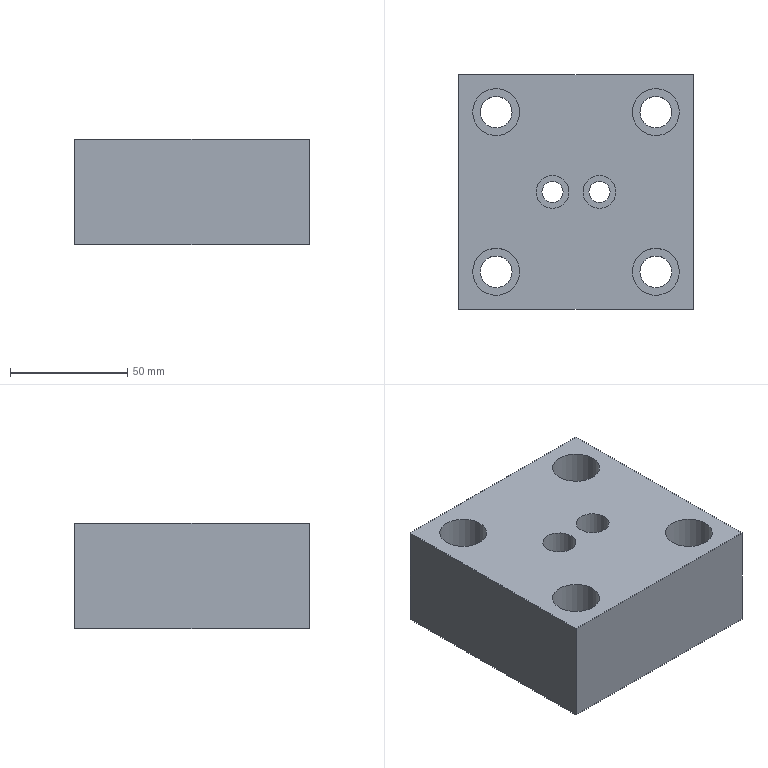Part | STEP file | lll_id554_x_t | 1 solid | 26 faces | box 100 x 100 x 45 mm | volume 329147 mm3 | plane 13 | cylinder 13 | commonest cylinder face diameters 13.509 x4 20.008 x4 9 x2 14 x2 65.2 x1
STEP:
#1=CARTESIAN_POINT('',(1525.035,-187.,246.5));
#2=VERTEX_POINT('',#1);
#3=CARTESIAN_POINT('',(1492.435,-187.,246.5));
#4=DIRECTION('',(0.,0.,1.));
#5=DIRECTION('',(1.,0.,0.));
#6=AXIS2_PLACEMENT_3D('',#3,#4,#5);
#7=CIRCLE('',#6,32.6);
#8=EDGE_CURVE('',#2,#2,#7,.T.);
#9=ORIENTED_EDGE('',*,*,#8,.F.);
#10=EDGE_LOOP('',(#9));
#11=FACE_BOUND('',#10,.T.);
#12=CARTESIAN_POINT('',(1486.935,-187.,246.5));
#13=VERTEX_POINT('',#12);
#14=CARTESIAN_POINT('',(1482.435,-187.,246.5));
#15=DIRECTION('',(0.,0.,1.));
#16=DIRECTION('',(1.,0.,0.));
#17=AXIS2_PLACEMENT_3D('',#14,#15,#16);
#18=CIRCLE('',#17,4.5);
#19=EDGE_CURVE('',#13,#13,#18,.T.);
#20=ORIENTED_EDGE('',*,*,#19,.T.);
#21=EDGE_LOOP('',(#20));
#22=FACE_BOUND('',#21,.T.);
#23=CARTESIAN_POINT('',(1506.935,-187.,246.5));
#24=VERTEX_POINT('',#23);
#25=CARTESIAN_POINT('',(1502.435,-187.,246.5));
#26=DIRECTION('',(0.,0.,-1.));
#27=DIRECTION('',(1.,0.,0.));
#28=AXIS2_PLACEMENT_3D('',#25,#26,#27);
#29=CIRCLE('',#28,4.5);
#30=EDGE_CURVE('',#24,#24,#29,.T.);
#31=ORIENTED_EDGE('',*,*,#30,.F.);
#32=EDGE_LOOP('',(#31));
#33=FACE_BOUND('',#32,.T.);
#34=CARTESIAN_POINT('',(1477.135,-187.,246.5));
#35=DIRECTION('',(0.,0.,1.));
#36=DIRECTION('',(1.,0.,0.));
#37=AXIS2_PLACEMENT_3D('',#34,#35,#36);
#38=PLANE('',#37);
#39=ADVANCED_FACE('',(#11,#22,#33),#38,.F.);
#40=CARTESIAN_POINT('',(1509.435,-187.,267.5));
#41=VERTEX_POINT('',#40);
#42=CARTESIAN_POINT('',(1502.435,-187.,267.5));
#43=DIRECTION('',(0.,0.,1.));
#44=DIRECTION('',(1.,0.,0.));
#45=AXIS2_PLACEMENT_3D('',#42,#43,#44);
#46=CIRCLE('',#45,7.);
#47=EDGE_CURVE('',#41,#41,#46,.T.);
#48=ORIENTED_EDGE('',*,*,#47,.F.);
#49=EDGE_LOOP('',(#48));
#50=FACE_BOUND('',#49,.T.);
#51=CARTESIAN_POINT('',(1489.435,-187.,267.5));
#52=VERTEX_POINT('',#51);
#53=CARTESIAN_POINT('',(1482.435,-187.,267.5));
#54=DIRECTION('',(0.,0.,1.));
#55=DIRECTION('',(1.,0.,0.));
#56=AXIS2_PLACEMENT_3D('',#53,#54,#55);
#57=CIRCLE('',#56,7.);
#58=EDGE_CURVE('',#52,#52,#57,.T.);
#59=ORIENTED_EDGE('',*,*,#58,.F.);
#60=EDGE_LOOP('',(#59));
#61=FACE_BOUND('',#60,.T.);
#62=CARTESIAN_POINT('',(1536.439,-153.,267.5));
#63=VERTEX_POINT('',#62);
#64=CARTESIAN_POINT('',(1526.435,-153.,267.5));
#65=DIRECTION('',(0.,0.,-1.));
#66=DIRECTION('',(1.,0.,0.));
#67=AXIS2_PLACEMENT_3D('',#64,#65,#66);
#68=CIRCLE('',#67,10.004);
#69=EDGE_CURVE('',#63,#63,#68,.T.);
#70=ORIENTED_EDGE('',*,*,#69,.T.);
#71=EDGE_LOOP('',(#70));
#72=FACE_BOUND('',#71,.T.);
#73=CARTESIAN_POINT('',(1468.439,-221.,267.5));
#74=VERTEX_POINT('',#73);
#75=CARTESIAN_POINT('',(1458.435,-221.,267.5));
#76=DIRECTION('',(0.,0.,-1.));
#77=DIRECTION('',(1.,0.,0.));
#78=AXIS2_PLACEMENT_3D('',#75,#76,#77);
#79=CIRCLE('',#78,10.004);
#80=EDGE_CURVE('',#74,#74,#79,.T.);
#81=ORIENTED_EDGE('',*,*,#80,.T.);
#82=EDGE_LOOP('',(#81));
#83=FACE_BOUND('',#82,.T.);
#84=CARTESIAN_POINT('',(1542.435,-137.,267.5));
#85=VERTEX_POINT('',#84);
#86=CARTESIAN_POINT('',(1542.435,-237.,267.5));
#87=VERTEX_POINT('',#86);
#88=CARTESIAN_POINT('',(1542.435,-187.,267.5));
#89=DIRECTION('',(0.,-1.,0.));
#90=VECTOR('',#89,1.);
#91=LINE('',#88,#90);
#92=EDGE_CURVE('',#85,#87,#91,.T.);
#93=ORIENTED_EDGE('',*,*,#92,.F.);
#94=CARTESIAN_POINT('',(1442.435,-137.,267.5));
#95=VERTEX_POINT('',#94);
#96=CARTESIAN_POINT('',(1492.435,-137.,267.5));
#97=DIRECTION('',(1.,0.,0.));
#98=VECTOR('',#97,1.);
#99=LINE('',#96,#98);
#100=EDGE_CURVE('',#95,#85,#99,.T.);
#101=ORIENTED_EDGE('',*,*,#100,.F.);
#102=CARTESIAN_POINT('',(1442.435,-237.,267.5));
#103=VERTEX_POINT('',#102);
#104=CARTESIAN_POINT('',(1442.435,-187.,267.5));
#105=DIRECTION('',(0.,1.,0.));
#106=VECTOR('',#105,1.);
#107=LINE('',#104,#106);
#108=EDGE_CURVE('',#103,#95,#107,.T.);
#109=ORIENTED_EDGE('',*,*,#108,.F.);
#110=CARTESIAN_POINT('',(1492.435,-237.,267.5));
#111=DIRECTION('',(-1.,0.,0.));
#112=VECTOR('',#111,1.);
#113=LINE('',#110,#112);
#114=EDGE_CURVE('',#87,#103,#113,.T.);
#115=ORIENTED_EDGE('',*,*,#114,.F.);
#116=EDGE_LOOP('',(#93,#101,#109,#115));
#117=FACE_BOUND('',#116,.T.);
#118=CARTESIAN_POINT('',(1468.439,-153.,267.5));
#119=VERTEX_POINT('',#118);
#120=CARTESIAN_POINT('',(1458.435,-153.,267.5));
#121=DIRECTION('',(0.,0.,-1.));
#122=DIRECTION('',(1.,0.,0.));
#123=AXIS2_PLACEMENT_3D('',#120,#121,#122);
#124=CIRCLE('',#123,10.004);
#125=EDGE_CURVE('',#119,#119,#124,.T.);
#126=ORIENTED_EDGE('',*,*,#125,.T.);
#127=EDGE_LOOP('',(#126));
#128=FACE_BOUND('',#127,.T.);
#129=CARTESIAN_POINT('',(1536.439,-221.,267.5));
#130=VERTEX_POINT('',#129);
#131=CARTESIAN_POINT('',(1526.435,-221.,267.5));
#132=DIRECTION('',(0.,0.,-1.));
#133=DIRECTION('',(1.,0.,0.));
#134=AXIS2_PLACEMENT_3D('',#131,#132,#133);
#135=CIRCLE('',#134,10.004);
#136=EDGE_CURVE('',#130,#130,#135,.T.);
#137=ORIENTED_EDGE('',*,*,#136,.T.);
#138=EDGE_LOOP('',(#137));
#139=FACE_BOUND('',#138,.T.);
#140=CARTESIAN_POINT('',(1492.435,-187.,267.5));
#141=DIRECTION('',(0.,0.,1.));
#142=DIRECTION('',(1.,0.,0.));
#143=AXIS2_PLACEMENT_3D('',#140,#141,#142);
#144=PLANE('',#143);
#145=ADVANCED_FACE('',(#50,#61,#72,#83,#117,#128,#139),#144,.T.);
#146=CARTESIAN_POINT('',(1525.035,-187.,222.5));
#147=VERTEX_POINT('',#146);
#148=CARTESIAN_POINT('',(1492.435,-187.,222.5));
#149=DIRECTION('',(0.,0.,1.));
#150=DIRECTION('',(1.,0.,0.));
#151=AXIS2_PLACEMENT_3D('',#148,#149,#150);
#152=CIRCLE('',#151,32.6);
#153=EDGE_CURVE('',#147,#147,#152,.T.);
#154=ORIENTED_EDGE('',*,*,#153,.F.);
#155=EDGE_LOOP('',(#154));
#156=FACE_BOUND('',#155,.T.);
#157=ORIENTED_EDGE('',*,*,#8,.T.);
#158=EDGE_LOOP('',(#157));
#159=FACE_BOUND('',#158,.T.);
#160=CARTESIAN_POINT('',(1492.435,-187.,246.5));
#161=DIRECTION('',(0.,0.,-1.));
#162=DIRECTION('',(-1.,0.,0.));
#163=AXIS2_PLACEMENT_3D('',#160,#161,#162);
#164=CYLINDRICAL_SURFACE('',#163,32.6);
#165=ADVANCED_FACE('',(#156,#159),#164,.F.);
#166=CARTESIAN_POINT('',(1442.435,-137.,222.5));
#167=VERTEX_POINT('',#166);
#168=CARTESIAN_POINT('',(1542.435,-137.,222.5));
#169=VERTEX_POINT('',#168);
#170=CARTESIAN_POINT('',(1492.435,-137.,222.5));
#171=DIRECTION('',(1.,0.,0.));
#172=VECTOR('',#171,1.);
#173=LINE('',#170,#172);
#174=EDGE_CURVE('',#167,#169,#173,.T.);
#175=ORIENTED_EDGE('',*,*,#174,.F.);
#176=CARTESIAN_POINT('',(1442.435,-137.,78.6));
#177=DIRECTION('',(0.,0.,1.));
#178=VECTOR('',#177,1.);
#179=LINE('',#176,#178);
#180=EDGE_CURVE('',#167,#95,#179,.T.);
#181=ORIENTED_EDGE('',*,*,#180,.T.);
#182=ORIENTED_EDGE('',*,*,#100,.T.);
#183=CARTESIAN_POINT('',(1542.435,-137.,78.6));
#184=DIRECTION('',(0.,0.,1.));
#185=VECTOR('',#184,1.);
#186=LINE('',#183,#185);
#187=EDGE_CURVE('',#169,#85,#186,.T.);
#188=ORIENTED_EDGE('',*,*,#187,.F.);
#189=EDGE_LOOP('',(#175,#181,#182,#188));
#190=FACE_OUTER_BOUND('',#189,.T.);
#191=CARTESIAN_POINT('',(1492.435,-137.,78.6));
#192=DIRECTION('',(0.,1.,0.));
#193=DIRECTION('',(0.,0.,1.));
#194=AXIS2_PLACEMENT_3D('',#191,#192,#193);
#195=PLANE('',#194);
#196=ADVANCED_FACE('',(#190),#195,.T.);
#197=CARTESIAN_POINT('',(1442.435,-237.,222.5));
#198=VERTEX_POINT('',#197);
#199=CARTESIAN_POINT('',(1442.435,-187.,222.5));
#200=DIRECTION('',(0.,1.,0.));
#201=VECTOR('',#200,1.);
#202=LINE('',#199,#201);
#203=EDGE_CURVE('',#198,#167,#202,.T.);
#204=ORIENTED_EDGE('',*,*,#203,.F.);
#205=CARTESIAN_POINT('',(1442.435,-237.,78.6));
#206=DIRECTION('',(0.,0.,1.));
#207=VECTOR('',#206,1.);
#208=LINE('',#205,#207);
#209=EDGE_CURVE('',#198,#103,#208,.T.);
#210=ORIENTED_EDGE('',*,*,#209,.T.);
#211=ORIENTED_EDGE('',*,*,#108,.T.);
#212=ORIENTED_EDGE('',*,*,#180,.F.);
#213=EDGE_LOOP('',(#204,#210,#211,#212));
#214=FACE_OUTER_BOUND('',#213,.T.);
#215=CARTESIAN_POINT('',(1442.435,-187.,78.6));
#216=DIRECTION('',(-1.,0.,0.));
#217=DIRECTION('',(0.,0.,1.));
#218=AXIS2_PLACEMENT_3D('',#215,#216,#217);
#219=PLANE('',#218);
#220=ADVANCED_FACE('',(#214),#219,.T.);
#221=CARTESIAN_POINT('',(1542.435,-237.,222.5));
#222=VERTEX_POINT('',#221);
#223=CARTESIAN_POINT('',(1492.435,-237.,222.5));
#224=DIRECTION('',(-1.,0.,0.));
#225=VECTOR('',#224,1.);
#226=LINE('',#223,#225);
#227=EDGE_CURVE('',#222,#198,#226,.T.);
#228=ORIENTED_EDGE('',*,*,#227,.F.);
#229=CARTESIAN_POINT('',(1542.435,-237.,78.6));
#230=DIRECTION('',(0.,0.,1.));
#231=VECTOR('',#230,1.);
#232=LINE('',#229,#231);
#233=EDGE_CURVE('',#222,#87,#232,.T.);
#234=ORIENTED_EDGE('',*,*,#233,.T.);
#235=ORIENTED_EDGE('',*,*,#114,.T.);
#236=ORIENTED_EDGE('',*,*,#209,.F.);
#237=EDGE_LOOP('',(#228,#234,#235,#236));
#238=FACE_OUTER_BOUND('',#237,.T.);
#239=CARTESIAN_POINT('',(1492.435,-237.,78.6));
#240=DIRECTION('',(0.,-1.,0.));
#241=DIRECTION('',(0.,0.,-1.));
#242=AXIS2_PLACEMENT_3D('',#239,#240,#241);
#243=PLANE('',#242);
#244=ADVANCED_FACE('',(#238),#243,.T.);
#245=CARTESIAN_POINT('',(1542.435,-187.,222.5));
#246=DIRECTION('',(0.,-1.,0.));
#247=VECTOR('',#246,1.);
#248=LINE('',#245,#247);
#249=EDGE_CURVE('',#169,#222,#248,.T.);
#250=ORIENTED_EDGE('',*,*,#249,.F.);
#251=ORIENTED_EDGE('',*,*,#187,.T.);
#252=ORIENTED_EDGE('',*,*,#92,.T.);
#253=ORIENTED_EDGE('',*,*,#233,.F.);
#254=EDGE_LOOP('',(#250,#251,#252,#253));
#255=FACE_OUTER_BOUND('',#254,.T.);
#256=CARTESIAN_POINT('',(1542.435,-187.,78.6));
#257=DIRECTION('',(1.,0.,0.));
#258=DIRECTION('',(0.,0.,-1.));
#259=AXIS2_PLACEMENT_3D('',#256,#257,#258);
#260=PLANE('',#259);
#261=ADVANCED_FACE('',(#255),#260,.T.);
#262=ORIENTED_EDGE('',*,*,#153,.T.);
#263=EDGE_LOOP('',(#262));
#264=FACE_BOUND('',#263,.T.);
#265=CARTESIAN_POINT('',(1533.19,-153.,222.5));
#266=VERTEX_POINT('',#265);
#267=CARTESIAN_POINT('',(1526.435,-153.,222.5));
#268=DIRECTION('',(0.,0.,1.));
#269=DIRECTION('',(1.,0.,0.));
#270=AXIS2_PLACEMENT_3D('',#267,#268,#269);
#271=CIRCLE('',#270,6.755);
#272=EDGE_CURVE('',#266,#266,#271,.T.);
#273=ORIENTED_EDGE('',*,*,#272,.T.);
#274=EDGE_LOOP('',(#273));
#275=FACE_BOUND('',#274,.T.);
#276=CARTESIAN_POINT('',(1533.19,-221.,222.5));
#277=VERTEX_POINT('',#276);
#278=CARTESIAN_POINT('',(1526.435,-221.,222.5));
#279=DIRECTION('',(0.,0.,1.));
#280=DIRECTION('',(1.,0.,0.));
#281=AXIS2_PLACEMENT_3D('',#278,#279,#280);
#282=CIRCLE('',#281,6.755);
#283=EDGE_CURVE('',#277,#277,#282,.T.);
#284=ORIENTED_EDGE('',*,*,#283,.T.);
#285=EDGE_LOOP('',(#284));
#286=FACE_BOUND('',#285,.T.);
#287=CARTESIAN_POINT('',(1465.19,-221.,222.5));
#288=VERTEX_POINT('',#287);
#289=CARTESIAN_POINT('',(1458.435,-221.,222.5));
#290=DIRECTION('',(0.,0.,1.));
#291=DIRECTION('',(1.,0.,0.));
#292=AXIS2_PLACEMENT_3D('',#289,#290,#291);
#293=CIRCLE('',#292,6.755);
#294=EDGE_CURVE('',#288,#288,#293,.T.);
#295=ORIENTED_EDGE('',*,*,#294,.T.);
#296=EDGE_LOOP('',(#295));
#297=FACE_BOUND('',#296,.T.);
#298=CARTESIAN_POINT('',(1465.19,-153.,222.5));
#299=VERTEX_POINT('',#298);
#300=CARTESIAN_POINT('',(1458.435,-153.,222.5));
#301=DIRECTION('',(0.,0.,1.));
#302=DIRECTION('',(1.,0.,0.));
#303=AXIS2_PLACEMENT_3D('',#300,#301,#302);
#304=CIRCLE('',#303,6.755);
#305=EDGE_CURVE('',#299,#299,#304,.T.);
#306=ORIENTED_EDGE('',*,*,#305,.T.);
#307=EDGE_LOOP('',(#306));
#308=FACE_BOUND('',#307,.T.);
#309=ORIENTED_EDGE('',*,*,#249,.T.);
#310=ORIENTED_EDGE('',*,*,#227,.T.);
#311=ORIENTED_EDGE('',*,*,#203,.T.);
#312=ORIENTED_EDGE('',*,*,#174,.T.);
#313=EDGE_LOOP('',(#309,#310,#311,#312));
#314=FACE_BOUND('',#313,.T.);
#315=CARTESIAN_POINT('',(3282.435,40.,222.5));
#316=DIRECTION('',(0.,0.,1.));
#317=DIRECTION('',(1.,0.,0.));
#318=AXIS2_PLACEMENT_3D('',#315,#316,#317);
#319=PLANE('',#318);
#320=ADVANCED_FACE('',(#264,#275,#286,#297,#308,#314),#319,.F.);
#321=CARTESIAN_POINT('',(1451.681,-153.,252.5));
#322=VERTEX_POINT('',#321);
#323=CARTESIAN_POINT('',(1458.435,-153.,252.5));
#324=DIRECTION('',(0.,0.,-1.));
#325=DIRECTION('',(-1.,0.,0.));
#326=AXIS2_PLACEMENT_3D('',#323,#324,#325);
#327=CIRCLE('',#326,6.755);
#328=EDGE_CURVE('',#322,#322,#327,.T.);
#329=ORIENTED_EDGE('',*,*,#328,.F.);
#330=EDGE_LOOP('',(#329));
#331=FACE_BOUND('',#330,.T.);
#332=ORIENTED_EDGE('',*,*,#305,.F.);
#333=EDGE_LOOP('',(#332));
#334=FACE_BOUND('',#333,.T.);
#335=CARTESIAN_POINT('',(1458.435,-153.,269.5));
#336=DIRECTION('',(0.,0.,-1.));
#337=DIRECTION('',(1.,0.,0.));
#338=AXIS2_PLACEMENT_3D('',#335,#336,#337);
#339=CYLINDRICAL_SURFACE('',#338,6.755);
#340=ADVANCED_FACE('',(#331,#334),#339,.F.);
#341=ORIENTED_EDGE('',*,*,#328,.T.);
#342=EDGE_LOOP('',(#341));
#343=FACE_BOUND('',#342,.T.);
#344=CARTESIAN_POINT('',(1468.439,-153.,252.5));
#345=VERTEX_POINT('',#344);
#346=CARTESIAN_POINT('',(1458.435,-153.,252.5));
#347=DIRECTION('',(0.,0.,-1.));
#348=DIRECTION('',(1.,0.,0.));
#349=AXIS2_PLACEMENT_3D('',#346,#347,#348);
#350=CIRCLE('',#349,10.004);
#351=EDGE_CURVE('',#345,#345,#350,.T.);
#352=ORIENTED_EDGE('',*,*,#351,.F.);
#353=EDGE_LOOP('',(#352));
#354=FACE_BOUND('',#353,.T.);
#355=CARTESIAN_POINT('',(1458.435,-153.,252.5));
#356=DIRECTION('',(0.,0.,-1.));
#357=DIRECTION('',(-1.,0.,0.));
#358=AXIS2_PLACEMENT_3D('',#355,#356,#357);
#359=PLANE('',#358);
#360=ADVANCED_FACE('',(#343,#354),#359,.F.);
#361=ORIENTED_EDGE('',*,*,#351,.T.);
#362=EDGE_LOOP('',(#361));
#363=FACE_BOUND('',#362,.T.);
#364=ORIENTED_EDGE('',*,*,#125,.F.);
#365=EDGE_LOOP('',(#364));
#366=FACE_BOUND('',#365,.T.);
#367=CARTESIAN_POINT('',(1458.435,-153.,267.5));
#368=DIRECTION('',(0.,0.,-1.));
#369=DIRECTION('',(1.,0.,0.));
#370=AXIS2_PLACEMENT_3D('',#367,#368,#369);
#371=CYLINDRICAL_SURFACE('',#370,10.004);
#372=ADVANCED_FACE('',(#363,#366),#371,.F.);
#373=CARTESIAN_POINT('',(1451.681,-221.,252.5));
#374=VERTEX_POINT('',#373);
#375=CARTESIAN_POINT('',(1458.435,-221.,252.5));
#376=DIRECTION('',(0.,0.,-1.));
#377=DIRECTION('',(-1.,0.,0.));
#378=AXIS2_PLACEMENT_3D('',#375,#376,#377);
#379=CIRCLE('',#378,6.755);
#380=EDGE_CURVE('',#374,#374,#379,.T.);
#381=ORIENTED_EDGE('',*,*,#380,.F.);
#382=EDGE_LOOP('',(#381));
#383=FACE_BOUND('',#382,.T.);
#384=ORIENTED_EDGE('',*,*,#294,.F.);
#385=EDGE_LOOP('',(#384));
#386=FACE_BOUND('',#385,.T.);
#387=CARTESIAN_POINT('',(1458.435,-221.,269.5));
#388=DIRECTION('',(0.,0.,-1.));
#389=DIRECTION('',(1.,0.,0.));
#390=AXIS2_PLACEMENT_3D('',#387,#388,#389);
#391=CYLINDRICAL_SURFACE('',#390,6.755);
#392=ADVANCED_FACE('',(#383,#386),#391,.F.);
#393=ORIENTED_EDGE('',*,*,#380,.T.);
#394=EDGE_LOOP('',(#393));
#395=FACE_BOUND('',#394,.T.);
#396=CARTESIAN_POINT('',(1468.439,-221.,252.5));
#397=VERTEX_POINT('',#396);
#398=CARTESIAN_POINT('',(1458.435,-221.,252.5));
#399=DIRECTION('',(0.,0.,-1.));
#400=DIRECTION('',(1.,0.,0.));
#401=AXIS2_PLACEMENT_3D('',#398,#399,#400);
#402=CIRCLE('',#401,10.004);
#403=EDGE_CURVE('',#397,#397,#402,.T.);
#404=ORIENTED_EDGE('',*,*,#403,.F.);
#405=EDGE_LOOP('',(#404));
#406=FACE_BOUND('',#405,.T.);
#407=CARTESIAN_POINT('',(1458.435,-221.,252.5));
#408=DIRECTION('',(0.,0.,-1.));
#409=DIRECTION('',(-1.,0.,0.));
#410=AXIS2_PLACEMENT_3D('',#407,#408,#409);
#411=PLANE('',#410);
#412=ADVANCED_FACE('',(#395,#406),#411,.F.);
#413=ORIENTED_EDGE('',*,*,#403,.T.);
#414=EDGE_LOOP('',(#413));
#415=FACE_BOUND('',#414,.T.);
#416=ORIENTED_EDGE('',*,*,#80,.F.);
#417=EDGE_LOOP('',(#416));
#418=FACE_BOUND('',#417,.T.);
#419=CARTESIAN_POINT('',(1458.435,-221.,267.5));
#420=DIRECTION('',(0.,0.,-1.));
#421=DIRECTION('',(1.,0.,0.));
#422=AXIS2_PLACEMENT_3D('',#419,#420,#421);
#423=CYLINDRICAL_SURFACE('',#422,10.004);
#424=ADVANCED_FACE('',(#415,#418),#423,.F.);
#425=CARTESIAN_POINT('',(1519.681,-221.,252.5));
#426=VERTEX_POINT('',#425);
#427=CARTESIAN_POINT('',(1526.435,-221.,252.5));
#428=DIRECTION('',(0.,0.,-1.));
#429=DIRECTION('',(-1.,0.,0.));
#430=AXIS2_PLACEMENT_3D('',#427,#428,#429);
#431=CIRCLE('',#430,6.755);
#432=EDGE_CURVE('',#426,#426,#431,.T.);
#433=ORIENTED_EDGE('',*,*,#432,.F.);
#434=EDGE_LOOP('',(#433));
#435=FACE_BOUND('',#434,.T.);
#436=ORIENTED_EDGE('',*,*,#283,.F.);
#437=EDGE_LOOP('',(#436));
#438=FACE_BOUND('',#437,.T.);
#439=CARTESIAN_POINT('',(1526.435,-221.,269.5));
#440=DIRECTION('',(0.,0.,-1.));
#441=DIRECTION('',(1.,0.,0.));
#442=AXIS2_PLACEMENT_3D('',#439,#440,#441);
#443=CYLINDRICAL_SURFACE('',#442,6.755);
#444=ADVANCED_FACE('',(#435,#438),#443,.F.);
#445=ORIENTED_EDGE('',*,*,#432,.T.);
#446=EDGE_LOOP('',(#445));
#447=FACE_BOUND('',#446,.T.);
#448=CARTESIAN_POINT('',(1536.439,-221.,252.5));
#449=VERTEX_POINT('',#448);
#450=CARTESIAN_POINT('',(1526.435,-221.,252.5));
#451=DIRECTION('',(0.,0.,-1.));
#452=DIRECTION('',(1.,0.,0.));
#453=AXIS2_PLACEMENT_3D('',#450,#451,#452);
#454=CIRCLE('',#453,10.004);
#455=EDGE_CURVE('',#449,#449,#454,.T.);
#456=ORIENTED_EDGE('',*,*,#455,.F.);
#457=EDGE_LOOP('',(#456));
#458=FACE_BOUND('',#457,.T.);
#459=CARTESIAN_POINT('',(1526.435,-221.,252.5));
#460=DIRECTION('',(0.,0.,-1.));
#461=DIRECTION('',(-1.,0.,0.));
#462=AXIS2_PLACEMENT_3D('',#459,#460,#461);
#463=PLANE('',#462);
#464=ADVANCED_FACE('',(#447,#458),#463,.F.);
#465=ORIENTED_EDGE('',*,*,#455,.T.);
#466=EDGE_LOOP('',(#465));
#467=FACE_BOUND('',#466,.T.);
#468=ORIENTED_EDGE('',*,*,#136,.F.);
#469=EDGE_LOOP('',(#468));
#470=FACE_BOUND('',#469,.T.);
#471=CARTESIAN_POINT('',(1526.435,-221.,267.5));
#472=DIRECTION('',(0.,0.,-1.));
#473=DIRECTION('',(1.,0.,0.));
#474=AXIS2_PLACEMENT_3D('',#471,#472,#473);
#475=CYLINDRICAL_SURFACE('',#474,10.004);
#476=ADVANCED_FACE('',(#467,#470),#475,.F.);
#477=CARTESIAN_POINT('',(1519.681,-153.,252.5));
#478=VERTEX_POINT('',#477);
#479=CARTESIAN_POINT('',(1526.435,-153.,252.5));
#480=DIRECTION('',(0.,0.,-1.));
#481=DIRECTION('',(-1.,0.,0.));
#482=AXIS2_PLACEMENT_3D('',#479,#480,#481);
#483=CIRCLE('',#482,6.755);
#484=EDGE_CURVE('',#478,#478,#483,.T.);
#485=ORIENTED_EDGE('',*,*,#484,.F.);
#486=EDGE_LOOP('',(#485));
#487=FACE_BOUND('',#486,.T.);
#488=ORIENTED_EDGE('',*,*,#272,.F.);
#489=EDGE_LOOP('',(#488));
#490=FACE_BOUND('',#489,.T.);
#491=CARTESIAN_POINT('',(1526.435,-153.,269.5));
#492=DIRECTION('',(0.,0.,-1.));
#493=DIRECTION('',(1.,0.,0.));
#494=AXIS2_PLACEMENT_3D('',#491,#492,#493);
#495=CYLINDRICAL_SURFACE('',#494,6.755);
#496=ADVANCED_FACE('',(#487,#490),#495,.F.);
#497=ORIENTED_EDGE('',*,*,#484,.T.);
#498=EDGE_LOOP('',(#497));
#499=FACE_BOUND('',#498,.T.);
#500=CARTESIAN_POINT('',(1536.439,-153.,252.5));
#501=VERTEX_POINT('',#500);
#502=CARTESIAN_POINT('',(1526.435,-153.,252.5));
#503=DIRECTION('',(0.,0.,-1.));
#504=DIRECTION('',(1.,0.,0.));
#505=AXIS2_PLACEMENT_3D('',#502,#503,#504);
#506=CIRCLE('',#505,10.004);
#507=EDGE_CURVE('',#501,#501,#506,.T.);
#508=ORIENTED_EDGE('',*,*,#507,.F.);
#509=EDGE_LOOP('',(#508));
#510=FACE_BOUND('',#509,.T.);
#511=CARTESIAN_POINT('',(1526.435,-153.,252.5));
#512=DIRECTION('',(0.,0.,-1.));
#513=DIRECTION('',(-1.,0.,0.));
#514=AXIS2_PLACEMENT_3D('',#511,#512,#513);
#515=PLANE('',#514);
#516=ADVANCED_FACE('',(#499,#510),#515,.F.);
#517=ORIENTED_EDGE('',*,*,#507,.T.);
#518=EDGE_LOOP('',(#517));
#519=FACE_BOUND('',#518,.T.);
#520=ORIENTED_EDGE('',*,*,#69,.F.);
#521=EDGE_LOOP('',(#520));
#522=FACE_BOUND('',#521,.T.);
#523=CARTESIAN_POINT('',(1526.435,-153.,267.5));
#524=DIRECTION('',(0.,0.,-1.));
#525=DIRECTION('',(1.,0.,0.));
#526=AXIS2_PLACEMENT_3D('',#523,#524,#525);
#527=CYLINDRICAL_SURFACE('',#526,10.004);
#528=ADVANCED_FACE('',(#519,#522),#527,.F.);
#529=CARTESIAN_POINT('',(1477.935,-187.,256.5));
#530=VERTEX_POINT('',#529);
#531=CARTESIAN_POINT('',(1482.435,-187.,256.5));
#532=DIRECTION('',(0.,0.,-1.));
#533=DIRECTION('',(-1.,0.,0.));
#534=AXIS2_PLACEMENT_3D('',#531,#532,#533);
#535=CIRCLE('',#534,4.5);
#536=EDGE_CURVE('',#530,#530,#535,.T.);
#537=ORIENTED_EDGE('',*,*,#536,.F.);
#538=EDGE_LOOP('',(#537));
#539=FACE_BOUND('',#538,.T.);
#540=ORIENTED_EDGE('',*,*,#19,.F.);
#541=EDGE_LOOP('',(#540));
#542=FACE_BOUND('',#541,.T.);
#543=CARTESIAN_POINT('',(1482.435,-187.,446.5));
#544=DIRECTION('',(0.,0.,-1.));
#545=DIRECTION('',(-1.,0.,0.));
#546=AXIS2_PLACEMENT_3D('',#543,#544,#545);
#547=CYLINDRICAL_SURFACE('',#546,4.5);
#548=ADVANCED_FACE('',(#539,#542),#547,.F.);
#549=CARTESIAN_POINT('',(1497.935,-187.,256.5));
#550=VERTEX_POINT('',#549);
#551=CARTESIAN_POINT('',(1502.435,-187.,256.5));
#552=DIRECTION('',(0.,0.,1.));
#553=DIRECTION('',(-1.,0.,0.));
#554=AXIS2_PLACEMENT_3D('',#551,#552,#553);
#555=CIRCLE('',#554,4.5);
#556=EDGE_CURVE('',#550,#550,#555,.T.);
#557=ORIENTED_EDGE('',*,*,#556,.T.);
#558=EDGE_LOOP('',(#557));
#559=FACE_BOUND('',#558,.T.);
#560=ORIENTED_EDGE('',*,*,#30,.T.);
#561=EDGE_LOOP('',(#560));
#562=FACE_BOUND('',#561,.T.);
#563=CARTESIAN_POINT('',(1502.435,-187.,446.5));
#564=DIRECTION('',(0.,0.,-1.));
#565=DIRECTION('',(-1.,0.,0.));
#566=AXIS2_PLACEMENT_3D('',#563,#564,#565);
#567=CYLINDRICAL_SURFACE('',#566,4.5);
#568=ADVANCED_FACE('',(#559,#562),#567,.F.);
#569=ORIENTED_EDGE('',*,*,#58,.T.);
#570=EDGE_LOOP('',(#569));
#571=FACE_BOUND('',#570,.T.);
#572=CARTESIAN_POINT('',(1475.435,-187.,256.5));
#573=VERTEX_POINT('',#572);
#574=CARTESIAN_POINT('',(1482.435,-187.,256.5));
#575=DIRECTION('',(0.,0.,1.));
#576=DIRECTION('',(-1.,0.,0.));
#577=AXIS2_PLACEMENT_3D('',#574,#575,#576);
#578=CIRCLE('',#577,7.);
#579=EDGE_CURVE('',#573,#573,#578,.T.);
#580=ORIENTED_EDGE('',*,*,#579,.F.);
#581=EDGE_LOOP('',(#580));
#582=FACE_BOUND('',#581,.T.);
#583=CARTESIAN_POINT('',(1482.435,-187.,446.5));
#584=DIRECTION('',(0.,0.,-1.));
#585=DIRECTION('',(-1.,0.,0.));
#586=AXIS2_PLACEMENT_3D('',#583,#584,#585);
#587=CYLINDRICAL_SURFACE('',#586,7.);
#588=ADVANCED_FACE('',(#571,#582),#587,.F.);
#589=ORIENTED_EDGE('',*,*,#536,.T.);
#590=EDGE_LOOP('',(#589));
#591=FACE_BOUND('',#590,.T.);
#592=ORIENTED_EDGE('',*,*,#579,.T.);
#593=EDGE_LOOP('',(#592));
#594=FACE_BOUND('',#593,.T.);
#595=CARTESIAN_POINT('',(1482.435,-187.,256.5));
#596=DIRECTION('',(0.,0.,-1.));
#597=DIRECTION('',(-1.,0.,0.));
#598=AXIS2_PLACEMENT_3D('',#595,#596,#597);
#599=PLANE('',#598);
#600=ADVANCED_FACE('',(#591,#594),#599,.F.);
#601=CARTESIAN_POINT('',(1495.435,-187.,256.5));
#602=VERTEX_POINT('',#601);
#603=CARTESIAN_POINT('',(1502.435,-187.,256.5));
#604=DIRECTION('',(0.,0.,1.));
#605=DIRECTION('',(-1.,0.,0.));
#606=AXIS2_PLACEMENT_3D('',#603,#604,#605);
#607=CIRCLE('',#606,7.);
#608=EDGE_CURVE('',#602,#602,#607,.T.);
#609=ORIENTED_EDGE('',*,*,#608,.T.);
#610=EDGE_LOOP('',(#609));
#611=FACE_BOUND('',#610,.T.);
#612=ORIENTED_EDGE('',*,*,#556,.F.);
#613=EDGE_LOOP('',(#612));
#614=FACE_BOUND('',#613,.T.);
#615=CARTESIAN_POINT('',(1502.435,-187.,256.5));
#616=DIRECTION('',(0.,0.,-1.));
#617=DIRECTION('',(-1.,0.,0.));
#618=AXIS2_PLACEMENT_3D('',#615,#616,#617);
#619=PLANE('',#618);
#620=ADVANCED_FACE('',(#611,#614),#619,.F.);
#621=ORIENTED_EDGE('',*,*,#47,.T.);
#622=EDGE_LOOP('',(#621));
#623=FACE_BOUND('',#622,.T.);
#624=ORIENTED_EDGE('',*,*,#608,.F.);
#625=EDGE_LOOP('',(#624));
#626=FACE_BOUND('',#625,.T.);
#627=CARTESIAN_POINT('',(1502.435,-187.,446.5));
#628=DIRECTION('',(0.,0.,-1.));
#629=DIRECTION('',(-1.,0.,0.));
#630=AXIS2_PLACEMENT_3D('',#627,#628,#629);
#631=CYLINDRICAL_SURFACE('',#630,7.);
#632=ADVANCED_FACE('',(#623,#626),#631,.F.);
#633=CLOSED_SHELL('',(#39,#145,#165,#196,#220,#244,#261,#320,#340,#360,#372,#392,#412,#424,#444,#464,#476,#496,#516,#528,#548,#568,#588,#600,#620,#632));
#634=MANIFOLD_SOLID_BREP('',#633);
#635=(LENGTH_UNIT()NAMED_UNIT(*)SI_UNIT(.MILLI.,.METRE.));
#636=UNCERTAINTY_MEASURE_WITH_UNIT(LENGTH_MEASURE(0.00002),#635,'','');
#637=(NAMED_UNIT(*)PLANE_ANGLE_UNIT()SI_UNIT($,.RADIAN.));
#638=PLANE_ANGLE_MEASURE_WITH_UNIT(PLANE_ANGLE_MEASURE(0.01745),#637);
#639=DIMENSIONAL_EXPONENTS(0.,0.,0.,0.,0.,0.,0.);
#640=(CONVERSION_BASED_UNIT('DEGREE',#638)NAMED_UNIT(#639)PLANE_ANGLE_UNIT());
#641=(NAMED_UNIT(*)SI_UNIT($,.STERADIAN.)SOLID_ANGLE_UNIT());
#642=(GEOMETRIC_REPRESENTATION_CONTEXT(3)GLOBAL_UNCERTAINTY_ASSIGNED_CONTEXT((#636))GLOBAL_UNIT_ASSIGNED_CONTEXT((#635,#640,#641))REPRESENTATION_CONTEXT('',''));
#643=ADVANCED_BREP_SHAPE_REPRESENTATION('',(#634),#642);